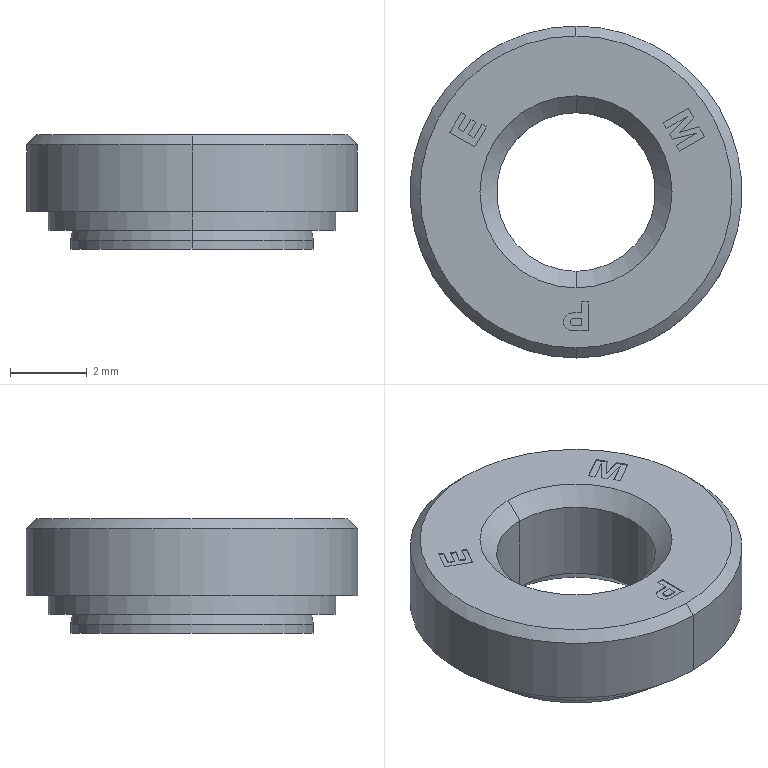Part | NX | features solid 2 | 1 solid | 59 faces | box 8.64 x 8.64 x 2.97 mm | volume 110.337 mm3 | plane 41 | cylinder 10 | cone 8 | commonest cylinder face diameters 4.134 x2 6.33 x2 7.485 x2 8.64 x2 0.196 x1 0.469 x1